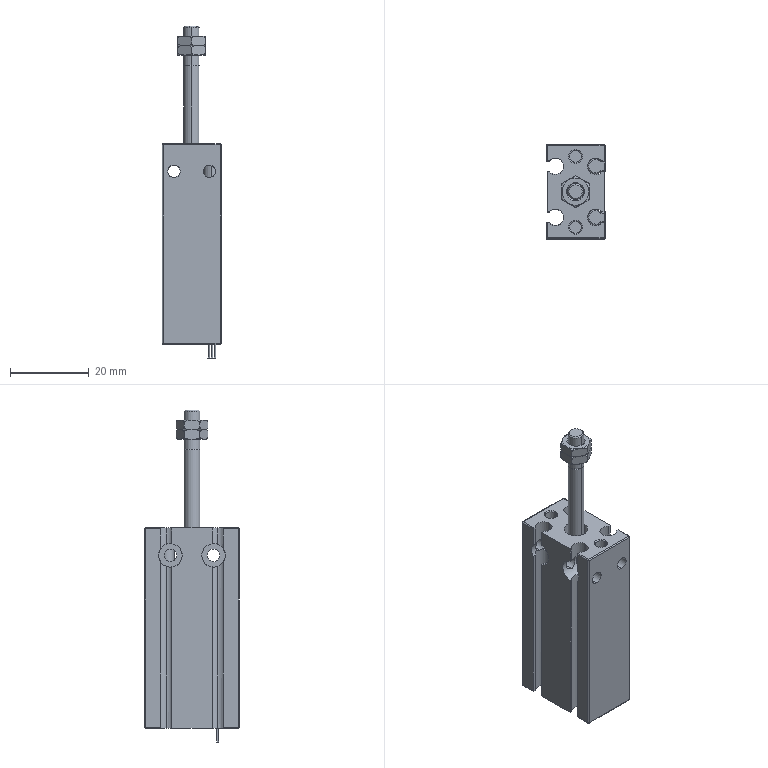Part | NX | 5 solids | 293 faces | box 15.21 x 24 x 84.5 mm | volume 13834 mm3 | cylinder 136 | plane 103 | torus 22 | cone 20 | sphere 8 | spline 4 | commonest cylinder face diameters 0.5 x28 3.2 x16 4 x14 6 x14 0.75 x12 4.2 x12